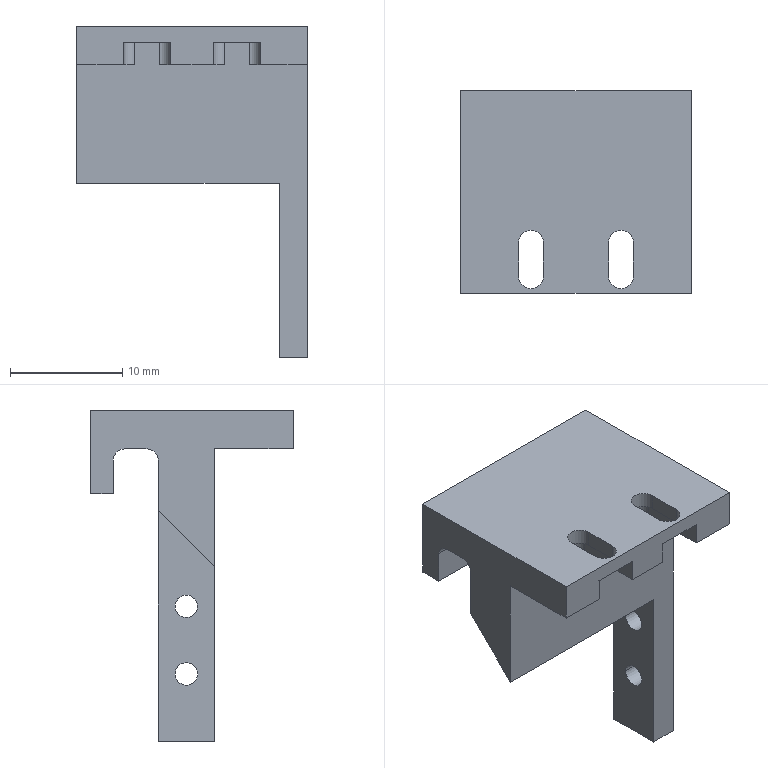NC program | NX | posted with a generic post | part box 20.5 x 18 x 29.4 mm
Lines 1801 to 1921 of 6588:
(11 , TOOL : D10JING)
N3594 T09 M6
N3596 G17 G43 G0 G90 X-17.059 Y-3.622 Z30. S9500 H9 M3
N3598 Z-5.333
N3600 G94 G1 Z-7.333 F1000.
N3602 X-15.75 Y-2.866
N3604 G3 X-15.25 Y-2. R1.
N3606 G1 Y3. F1200.
N3608 G2 X-10.25 Y8. R5.
N3610 G1 X-7.75
N3612 G2 X-2.75 Y3. R5.
N3614 G1 Y-2.
N3616 G2 X-7.75 Y-7. R5.
N3618 G1 X-10.25
N3620 G2 X-15.25 Y-2. R5.
N3622 G3 X-15.75 Y-1.134 R1.
N3624 G1 X-17.25 Y-0.268
N3626 Z-5.333
N3628 G0 Z30.
N3630 X-17.059 Y-3.622
N3632 Z-12.667
N3634 G1 Z-14.667 F1000.
N3636 X-15.75 Y-2.866
N3638 G3 X-15.25 Y-2. R1.
N3640 G1 Y3. F1200.
N3642 G2 X-10.25 Y8. R5.
N3644 G1 X-7.75
N3646 G2 X-2.75 Y3. R5.
N3648 G1 Y-2.
N3650 G2 X-7.75 Y-7. R5.
N3652 G1 X-10.25
N3654 G2 X-15.25 Y-2. R5.
N3656 G3 X-15.75 Y-1.134 R1.
N3658 G1 X-17.25 Y-0.268
N3660 Z-12.667
N3662 G0 Z30.
N3664 X-17.059 Y-3.622
N3666 Z-20.
N3668 G1 Z-22. F1000.
N3670 X-15.75 Y-2.866
N3672 G3 X-15.25 Y-2. R1.
N3674 G1 Y3. F1200.
N3676 G2 X-10.25 Y8. R5.
N3678 G1 X10.25
N3680 G2 X15.25 Y3. R5.
N3682 G1 Y-2.
N3684 G2 X10.25 Y-7. R5.
N3686 G1 X-10.25
N3688 G2 X-15.25 Y-2. R5.
N3690 G3 X-15.75 Y-1.134 R1.
N3692 G1 X-17.25 Y-0.268
N3694 Z-20.
N3696 G0 Z30.
N3698 X-17.059 Y-3.622
N3700 Z-24.
N3702 G1 Z-26. F1000.
N3704 X-15.75 Y-2.866
N3706 G3 X-15.25 Y-2. R1.
N3708 G1 Y3.962 F1200.
N3710 G2 X-15.134 Y4.997 R4.942
N3712 X-15.25 Y6.038 R5.177
N3714 G1 Y9.
N3716 G2 X-10.25 Y14. R5.
N3718 G1 X10.25
N3720 G2 X15.25 Y9. R5.
N3722 G1 Y6.038
N3724 G2 X15.133 Y4.999 R5.116
N3726 X15.25 Y3.962 R5.009
N3728 G1 Y-2.
N3730 G2 X10.25 Y-7. R5.
N3732 G1 X-10.25
N3734 G2 X-15.25 Y-2. R5.
N3736 G3 X-15.75 Y-1.134 R1.
N3738 G1 X-17.25 Y-0.268
N3740 Z-24.
N3742 G0 Z30.
N3744 Y-3.732
N3746 Z-26.
N3748 G1 Z-28. F1000.
N3750 X-15.75 Y-2.866
N3752 G3 X-15.25 Y-2. R1.
N3754 G1 Y9. F1200.
N3756 G2 X-10.25 Y14. R5.
N3758 G1 X10.25
N3760 G2 X15.25 Y9. R5.
N3762 G1 Y-9.
N3764 G2 X10.25 Y-14. R5.
N3766 G1 X6.1
N3768 G2 X4. Y-13.538 R5.
N3770 X1.9 Y-14. R5.
N3772 G1 X-1.9
N3774 G2 X-4. Y-13.538 R5.
N3776 X-6.1 Y-14. R5.
N3778 G1 X-10.25
N3780 G2 X-15.25 Y-9. R5.
N3782 G1 Y-2.
N3784 G3 X-15.75 Y-1.134 R1.
N3786 G1 X-17.25 Y-0.268
N3788 Z-26.
N3790 G0 Z30.
N3792 Y-3.732
N3794 Z-27.25
N3796 G1 Z-29.25 F1000.
N3798 X-15.75 Y-2.866
N3800 G3 X-15.25 Y-2. R1.
N3802 G1 Y9. F1200.
N3804 G2 X-10.25 Y14. R5.
N3806 G1 X10.25
N3808 G2 X15.25 Y9. R5.
N3810 G1 Y-9.
N3812 G2 X10.25 Y-14. R5.
N3814 G1 X-10.25
N3816 G2 X-15.25 Y-9. R5.
N3818 G1 Y-2.
N3820 G3 X-15.75 Y-1.134 R1.
N3822 G1 X-17.25 Y-0.268
N3824 Z-27.25
N3826 G0 Z30.
N3828 M5